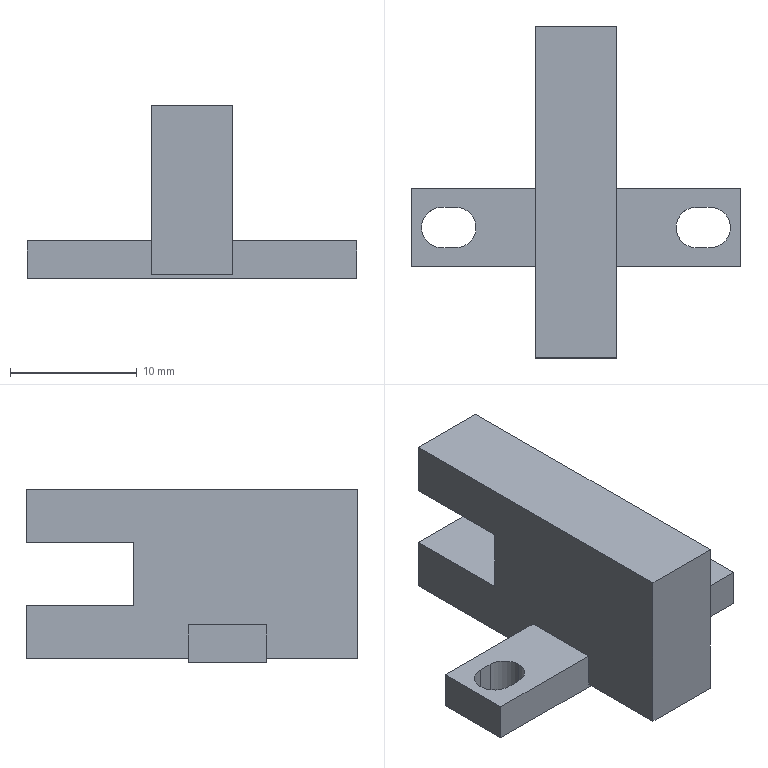Part | STEP file | FC-SPX303Z | 1 solid | 28 faces | box 26 x 26.2 x 13.7 mm | volume 2282 mm3 | plane 22 | cylinder 6 | commonest cylinder face diameters 3.2 x6